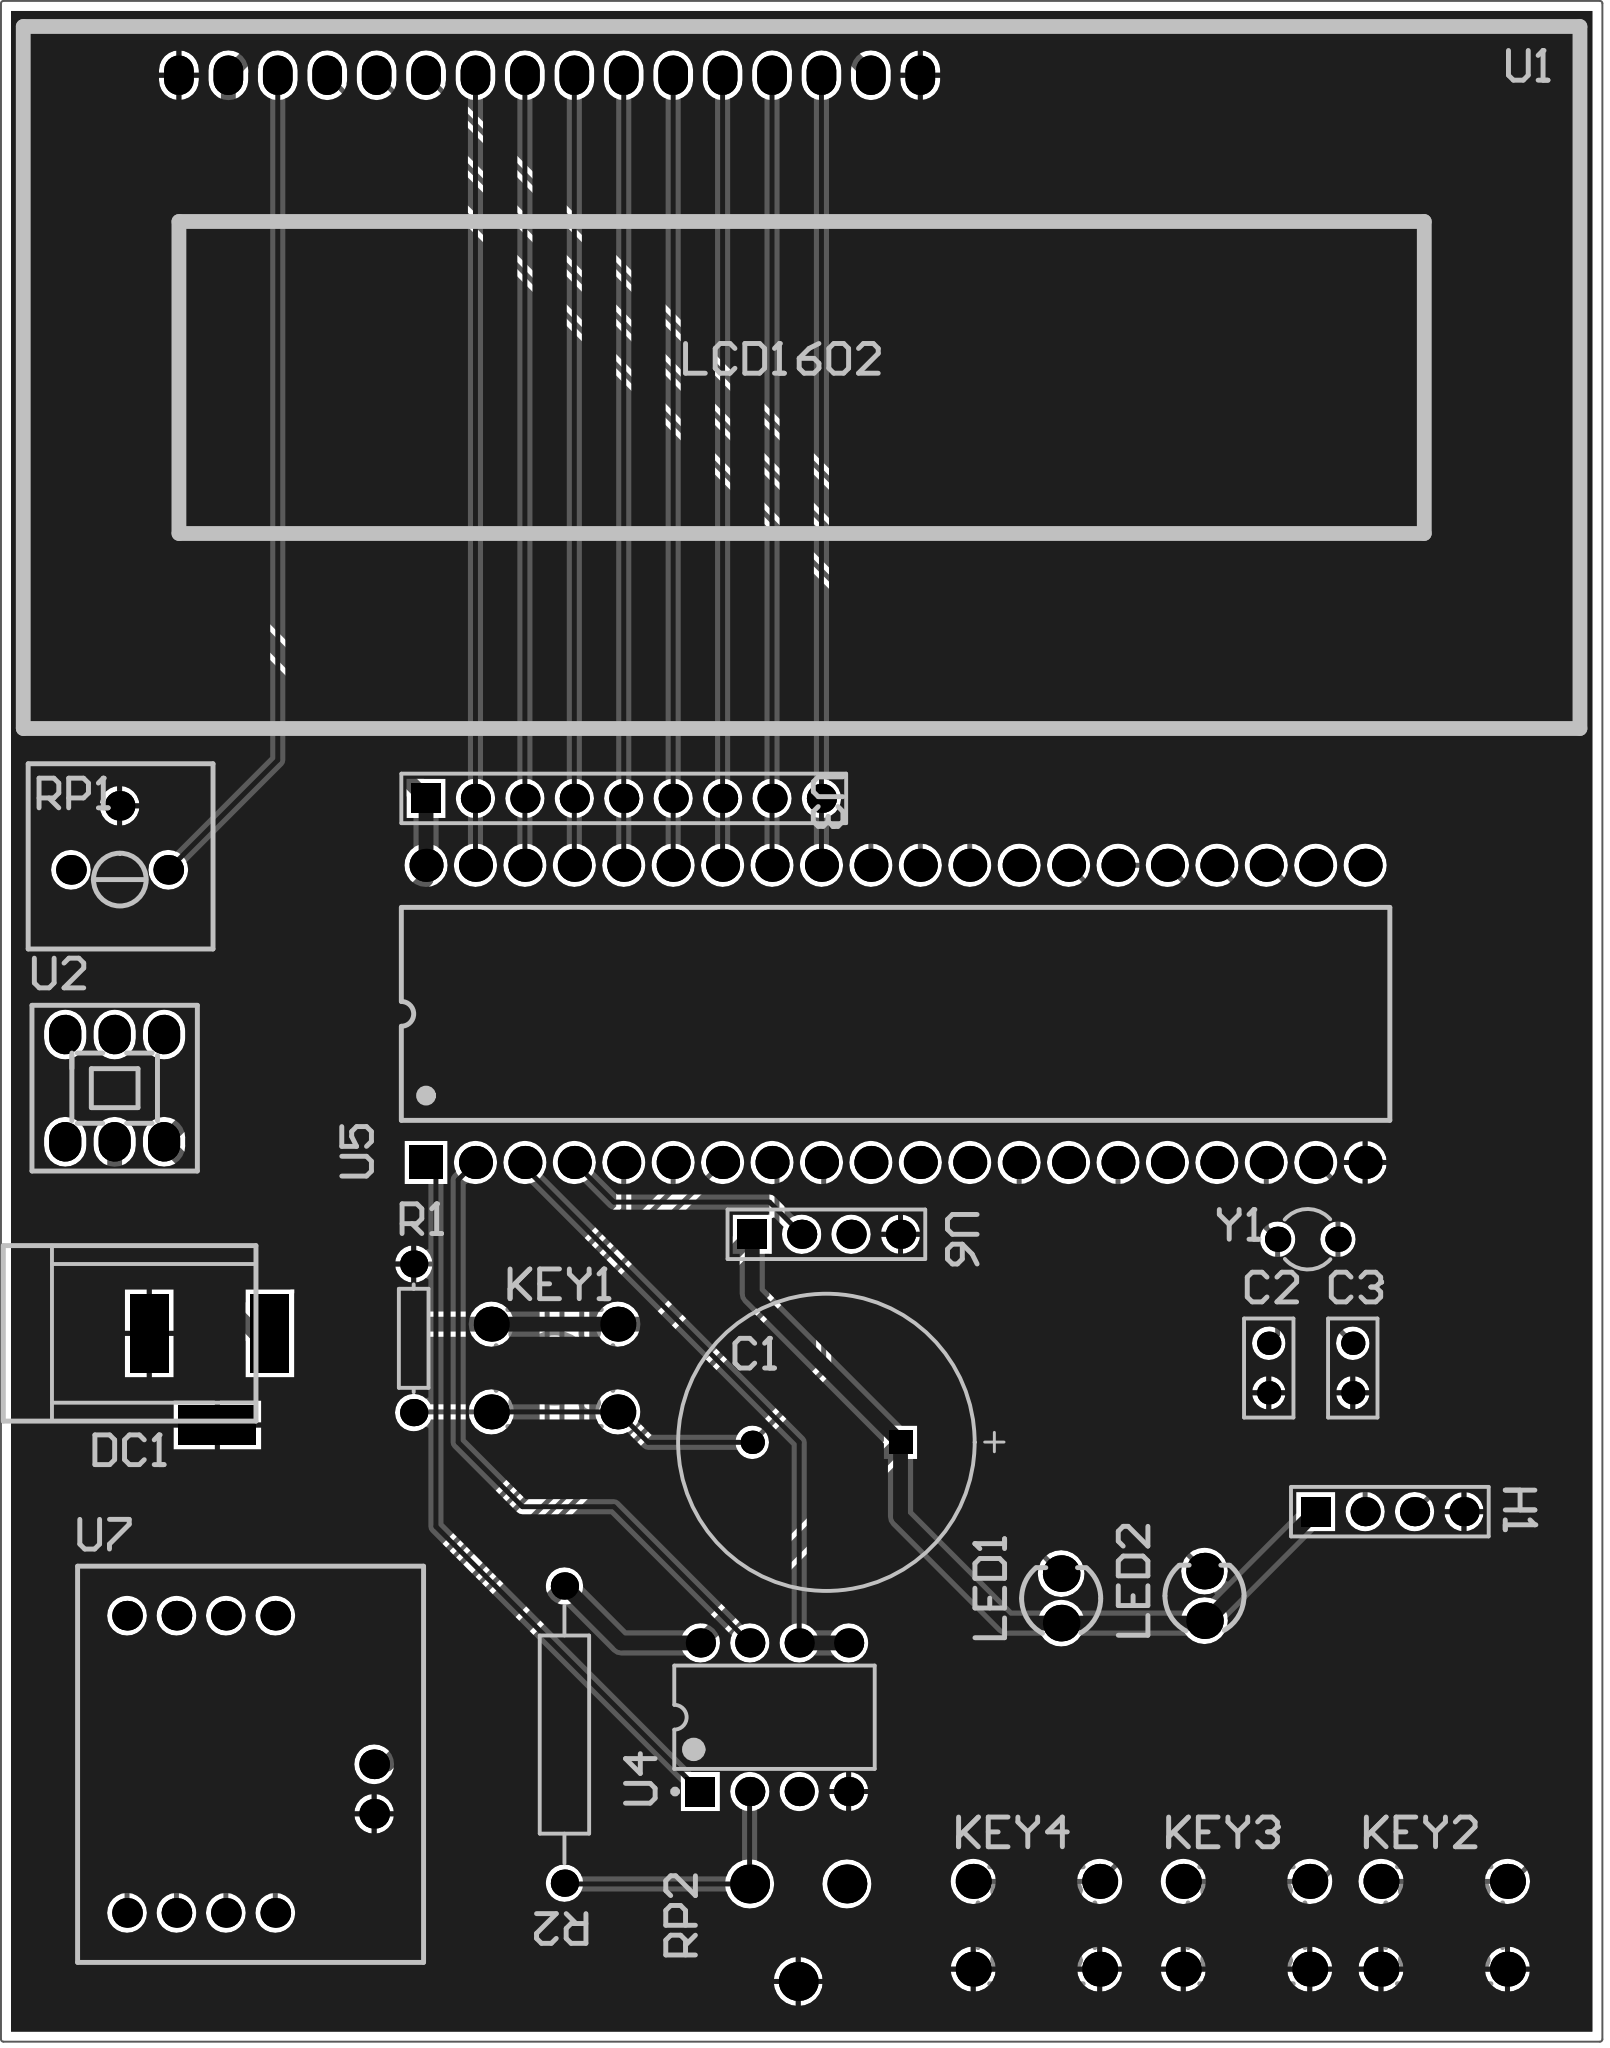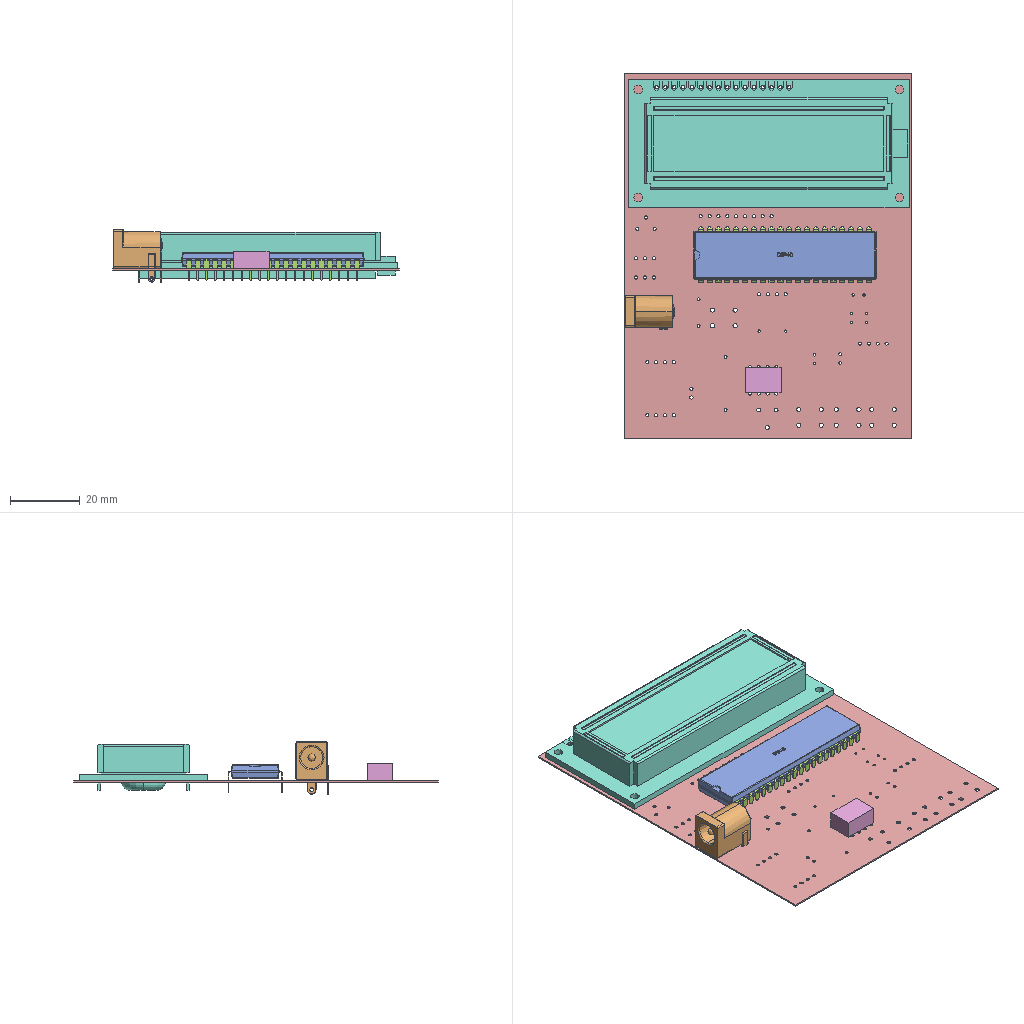Circuit board layout | Altium Designer | box 82.3 x 104.6 x 15 mm
Layer stack:
# Altium Designer layer stack of  (unit mm; dielectric type: 0 none, 1 core, 2 prepreg, 3 surface material)
index,name,kind,layer,copper_thickness_mm,dielectric_type,dielectric_thickness_mm,dielectric_material,dielectric_constant
0,Top Paste,other,,,,,,
1,Top Overlay,other,,,,,,
2,Top Solder,dielectric,,,3,0.0102,Solder Resist,3.5
3,Top Layer,copper,Top Layer,0.0356,,,,
4,Dielectric 1,dielectric,,,0,0.32,FR-4,4.8
5,Bottom Layer,copper,Bottom Layer,0.0356,,,,
6,Bottom Solder,dielectric,,,3,0.0102,Solder Resist,3.5
7,Bottom Overlay,other,,,,,,
8,Bottom Paste,other,,,,,,
# drill layer pairs: low layer,high layer
drill_pair,Top Layer,Bottom Layer
Part placement:
Designator,Comment,Layer,Footprint,Center-X(mm),Center-Y(mm),Rotation
Y1,12M,TopLayer,R38,114.02,63.627,270
U7,ULN2003 stepper motor driver,TopLayer,ULN2003,59.69,36.703,90
U6,DHT11,TopLayer,HDR1X4,89.281,63.881,360
U5,STC89C52RC,TopLayer,DIP40,92.837,75.184,90
U4,ADC0832,TopLayer,DIP-8,86.614,39.116,90
U3,respack-8,TopLayer,HDR1X9,78.867,86.233,360
U2,Self-locking switch_power supply,TopLayer,自锁开关,52.705,71.374,0
U1,1602,TopLayer,LCD1602,75.057,123.317,360
RP2,103,TopLayer,RM065,87.834,28.068,180
RP1,502,TopLayer,电位器,52.959,84.211,0
R2,Photoresistor,TopLayer,AXIAL-0.6,75.819,38.227,270
R1,10k,TopLayer,AXIAL-0.3,68.072,58.547,90
LED2,LED-0603_R,TopLayer,LED3MM,108.712,45.339,90
LED1,LED-0603_R,TopLayer,LED3MM,101.346,45.212,90
KEY4,button6*6*8.5,TopLayer,四脚轻触开关,100.076,28.448,0
KEY3,button6*6*8.5,TopLayer,四脚轻触开关,110.871,28.448,0
KEY2,button6*6*8.5,TopLayer,四脚轻触开关,121.031,28.448,0
KEY1,button6*6*8.5,TopLayer,四脚轻触开关,75.311,57.023,180
H1,Pressure sensor,TopLayer,HDR1X4,118.237,49.657,360
DC1,DC-005,TopLayer,DC-005,57.583,56.451,180
C3,33p,TopLayer,RAD-0.1,116.332,57.023,90
C2,33p,TopLayer,RAD-0.1,112.014,57.023,90
C1,10uF,TopLayer,RB7.6-15,89.281,53.213,0
Pad and via stacks:
# Altium Designer via and pad stacks of  (unit mm). Each distinct definition once, with the count of objects using it.
# via: kind,start_layer,end_layer,hole_mm,diameter_mm,mode(0 simple;1 top-mid-bottom;2 full stack),diameter_per_layer,count,example_net
# pad: kind,layer,hole_mm,hole_type(0 round;1 square;2 slot),plating,top_size,top_shape(1 round;2 rect;3 octagon;9 rounded rect),mid_size,bottom_size,mode,footprint,size_per_layer,count,example
pad,Multi-Layer,0.9,0,plated,1.5x1.5,2,1.5x1.5,1.5x1.5,0,HDR1X9,,1,U3.1
pad,Multi-Layer,0.9,0,plated,1.5x1.5,1,1.5x1.5,1.5x1.5,0,HDR1X9,,8,U3.3
pad,Multi-Layer,0.9,0,plated,1.524x2.032,1,1.524x2.032,1.524x2.032,0,LCD1602,,16,U1.1
pad,Multi-Layer,0.8,2,plated,2x4,2,2x4,2x4,0,DC-005,,2,DC1.1
pad,Multi-Layer,0.8,2,plated,4x2,2,4x2,4x2,0,DC-005,,1,DC1.3
pad,Multi-Layer,0.9144,0,plated,1.651x2.032,1,1.651x2.032,1.651x2.032,0,\u00D7\u00D4\u00CB\u00F8\u00BF\u00AA\u00B9\u00D8,,6,U2.6
pad,Multi-Layer,0.9,0,plated,1.5x1.5,1,1.5x1.5,1.5x1.5,0,HDR1X4,,6,U6.4
pad,Multi-Layer,0.9,0,plated,1.5x1.5,2,1.5x1.5,1.5x1.5,0,HDR1X4,,2,U6.1
pad,Multi-Layer,0.9,0,plated,1.524x1.524,1,1.524x1.524,1.524x1.524,0,\u00B5\u00E7\u00CE\u00BB\u00C6\u00F7,,3,RP1.3
pad,Multi-Layer,0.85,0,plated,1.4x1.4,1,1.4x1.4,1.4x1.4,0,AXIAL-0.6,,2,R2.2
pad,Multi-Layer,0.8,0,plated,1.7x1.7,1,1.7x1.7,1.7x1.7,0,DIP40,,39,U5.21
pad,Multi-Layer,0.8,0,plated,1.7x1.7,2,1.7x1.7,1.7x1.7,0,DIP40,,1,U5.1
pad,Multi-Layer,0.9,0,plated,1.5x1.5,2,1.5x1.5,1.5x1.5,0,DIP-8,,1,U4.1
pad,Multi-Layer,0.9,0,plated,1.5x1.5,1,1.5x1.5,1.5x1.5,0,DIP-8,,7,U4.2
pad,Multi-Layer,1.1,0,plated,2x2,1,2x2,2x2,0,RM065,,3,RP2.1
pad,Multi-Layer,0.85,0,plated,1.4x1.4,1,1.4x1.4,1.4x1.4,0,AXIAL-0.3,,2,R1.2
pad,Multi-Layer,0.8128,2,plated,1.88x1.88,1,1.88x1.88,1.88x1.88,0,LED3MM,,4,LED2.2
pad,Multi-Layer,1.2,0,plated,1.8x1.8,1,1.8x1.8,1.8x1.8,0,\u00CB\u00C4\u00BD\u00C5\u00C7\u00E1\u00B4\u00A5\u00BF\u00AA\u00B9\u00D8,,16,KEY1.4
pad,Multi-Layer,0.7,0,plated,1.2x1.2,2,1.2x1.2,1.2x1.2,0,RB7.6-15,,1,C1.1
pad,Multi-Layer,0.7,0,plated,1.2x1.2,1,1.2x1.2,1.2x1.2,0,RB7.6-15,,1,C1.2
pad,Multi-Layer,0.7,0,plated,1.3x1.3,1,1.3x1.3,1.3x1.3,0,R38,,2,Y1.1
pad,Multi-Layer,0.7,0,plated,1.2x1.2,1,1.2x1.2,1.2x1.2,0,RAD-0.1,,4,C2.1
pad,Multi-Layer,0.9144,0,plated,1.524x1.524,1,1.524x1.524,1.524x1.524,0,ULN2003,,10,U7.10
Copper pours:
name,layer,net,type(0 solid;1 hatched;2 none)
G,Bottom Layer,GND,0
G,Top Layer,GND,0
Design rules, without the lines most boards share:
# Altium Designer design rules of  (exported by Altium Designer, unit mm)
# columns: name | kind | enabled | priority | scope1 | scope2 | descriptor | typed fields (field=value)
SilkToSilkClearance | 55 | enabled | 1 | All | All | Silk to Silk (Clearance=0mil) (All),(All) |
SilkToSolderMaskClearance | 54 | enabled | 1 | IsPad | All | Silk To Solder Mask (Clearance=0mil) (IsPad),(All) |
MinimumSolderMaskSliver | 53 | enabled | 1 | All | All | Minimum Solder Mask Sliver (Gap=0mil) (All),(All) |
HoleToHoleClearance | 52 | enabled | 1 | All | All | Hole To Hole Clearance (Gap=10mil) (All),(All) | gap=0.254
DiffPairsRouting | 51 | enabled | 1 | All | All | Differential Pairs Uncoupled Length using the Gap Constraints (Min=10mil) (Max=10mil) (Prefered=10mil)  and Width Constraints (Min=15mil) (Max=15mil) (Prefered=15mil) (All) |
SolderMaskExpansion | 13 | enabled | 1 | All | All | Solder Mask Expansion (Expansion =4mil) (All) | expansion=0.1016
PasteMaskExpansion | 14 | enabled | 1 | All | All | Paste Mask Expansion (Expansion =0mil) (All) | expansion=0
RoutingVias | 11 | enabled | 1 | All | All | Routing Via (MinHoleWidth=28mil) (MaxHoleWidth=28mil) (PreferredHoleWidth=28mil) (MinWidth=50mil) (MaxWidth=50mil) (PreferedWidth=50mil) (All) | via_min_hole=0.7112 via_max_hole=0.7112 via_preferred_diameter=1.27 via_preferred_hole=0.7112
Width | 2 | enabled | 1 | All | All | Width Constraint (Min=10mil) (Max=30mil) (Preferred=10mil) (All) |
PolygonConnect | 20 | enabled | 1 | All | All | Polygon Connect Rule(Relief Connect )(Conductor Width=10mil) (Relief Angle=90 Angle) (Entries=4) (Air Gap Width=10mil) (All),(All) | connect_style(0=relief,1=direct,2=none)=0 relief_conductor_width=0.254 relief_entries=4
PlaneConnect | 6 | enabled | 1 | All | All | Power Plane Connect Rule(Relief Connect )(Expansion=20mil) (Conductor Width=10mil) (Air Gap=10mil) (Entries=4) (All) | relief_conductor_width=0.254 relief_entries=4 relief_expansion=0.508
Clearance | 0 | enabled | 1 | All | All | Clearance Constraint (Gap=10mil) (All),(All) | gap=0.254